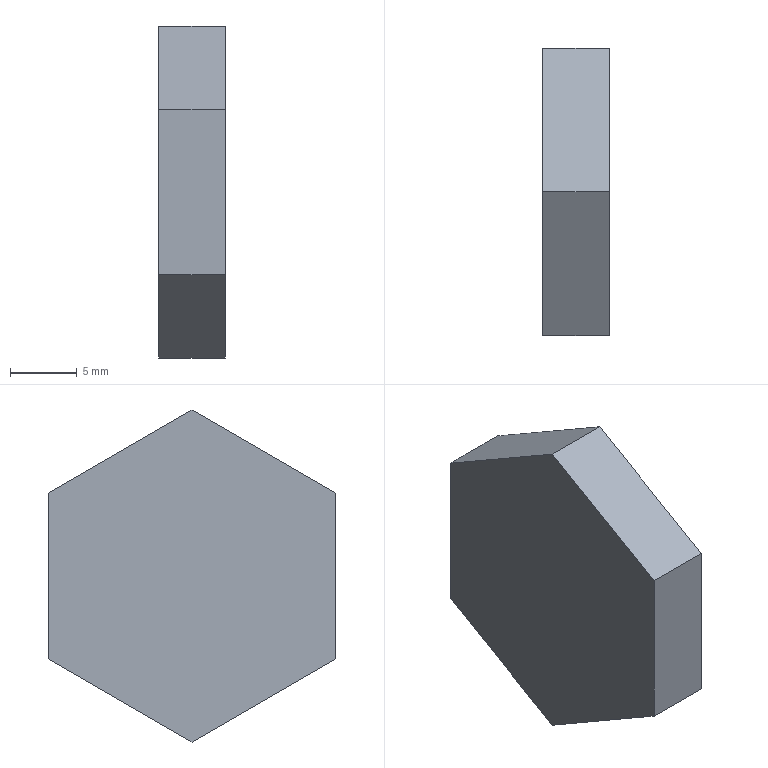Part | STEP file | 1 solid | 8 faces | box 5 x 21.5 x 24.826 mm | volume 2002 mm3 | plane 8
STEP:
#1=CARTESIAN_POINT('',(0.,0.,0.));
#2=DIRECTION('',(0.,0.,1.));
#3=DIRECTION('',(1.,0.,0.));
#4=AXIS2_PLACEMENT_3D('',#1,#2,#3);
#5=CARTESIAN_POINT('',(-24.,-10.75,6.207));
#6=VERTEX_POINT('',#5);
#7=CARTESIAN_POINT('',(-24.,-10.75,-6.207));
#8=VERTEX_POINT('',#7);
#9=CARTESIAN_POINT('',(-24.,-10.75,6.207));
#10=DIRECTION('',(0.,0.,-1.));
#11=VECTOR('',#10,1.);
#12=LINE('',#9,#11);
#13=CARTESIAN_POINT('',(-29.,-10.75,-3.464));
#14=DIRECTION('',(0.,1.,0.));
#15=DIRECTION('',(0.,0.,1.));
#16=AXIS2_PLACEMENT_3D('',#13,#14,#15);
#17=PLANE('',#16);
#18=CARTESIAN_POINT('',(9.671,5.));
#19=DIRECTION('',(-1.,0.));
#20=VECTOR('',#19,1.);
#21=LINE('',#18,#20);
#22=(GEOMETRIC_REPRESENTATION_CONTEXT(2)PARAMETRIC_REPRESENTATION_CONTEXT()REPRESENTATION_CONTEXT('',''));
#23=DEFINITIONAL_REPRESENTATION('',(#21),#22);
#24=PCURVE('',#17,#23);
#25=CARTESIAN_POINT('',(-24.,55.,0.));
#26=DIRECTION('',(-1.,0.,0.));
#27=DIRECTION('',(0.,0.,1.));
#28=AXIS2_PLACEMENT_3D('',#25,#26,#27);
#29=PLANE('',#28);
#30=CARTESIAN_POINT('',(6.207,-65.75));
#31=DIRECTION('',(-1.,0.));
#32=VECTOR('',#31,1.);
#33=LINE('',#30,#32);
#34=(GEOMETRIC_REPRESENTATION_CONTEXT(2)PARAMETRIC_REPRESENTATION_CONTEXT()REPRESENTATION_CONTEXT('',''));
#35=DEFINITIONAL_REPRESENTATION('',(#33),#34);
#36=PCURVE('',#29,#35);
#37=SURFACE_CURVE('',#12,(#24,#36),.PCURVE_S1.);
#38=EDGE_CURVE('',#6,#8,#37,.T.);
#39=ORIENTED_EDGE('',*,*,#38,.T.);
#40=CARTESIAN_POINT('',(-29.,-10.75,-6.207));
#41=VERTEX_POINT('',#40);
#42=CARTESIAN_POINT('',(-24.,-10.75,-6.207));
#43=DIRECTION('',(-1.,0.,0.));
#44=VECTOR('',#43,1.);
#45=LINE('',#42,#44);
#46=CARTESIAN_POINT('',(-2.742,5.));
#47=DIRECTION('',(0.,-1.));
#48=VECTOR('',#47,1.);
#49=LINE('',#46,#48);
#50=(GEOMETRIC_REPRESENTATION_CONTEXT(2)PARAMETRIC_REPRESENTATION_CONTEXT()REPRESENTATION_CONTEXT('',''));
#51=DEFINITIONAL_REPRESENTATION('',(#49),#50);
#52=PCURVE('',#17,#51);
#53=CARTESIAN_POINT('',(-29.,-2.375,-11.042));
#54=DIRECTION('',(0.,0.5,0.866));
#55=DIRECTION('',(0.,-0.866,0.5));
#56=AXIS2_PLACEMENT_3D('',#53,#54,#55);
#57=PLANE('',#56);
#58=CARTESIAN_POINT('',(9.671,5.));
#59=DIRECTION('',(0.,-1.));
#60=VECTOR('',#59,1.);
#61=LINE('',#58,#60);
#62=(GEOMETRIC_REPRESENTATION_CONTEXT(2)PARAMETRIC_REPRESENTATION_CONTEXT()REPRESENTATION_CONTEXT('',''));
#63=DEFINITIONAL_REPRESENTATION('',(#61),#62);
#64=PCURVE('',#57,#63);
#65=SURFACE_CURVE('',#45,(#52,#64),.PCURVE_S1.);
#66=EDGE_CURVE('',#8,#41,#65,.T.);
#67=ORIENTED_EDGE('',*,*,#66,.T.);
#68=CARTESIAN_POINT('',(-29.,-10.75,6.207));
#69=VERTEX_POINT('',#68);
#70=CARTESIAN_POINT('',(-29.,-10.75,6.207));
#71=DIRECTION('',(0.,0.,-1.));
#72=VECTOR('',#71,1.);
#73=LINE('',#70,#72);
#74=CARTESIAN_POINT('',(9.671,0.));
#75=DIRECTION('',(-1.,0.));
#76=VECTOR('',#75,1.);
#77=LINE('',#74,#76);
#78=(GEOMETRIC_REPRESENTATION_CONTEXT(2)PARAMETRIC_REPRESENTATION_CONTEXT()REPRESENTATION_CONTEXT('',''));
#79=DEFINITIONAL_REPRESENTATION('',(#77),#78);
#80=PCURVE('',#17,#79);
#81=CARTESIAN_POINT('',(-29.,55.,0.));
#82=DIRECTION('',(-1.,0.,0.));
#83=DIRECTION('',(0.,0.,1.));
#84=AXIS2_PLACEMENT_3D('',#81,#82,#83);
#85=PLANE('',#84);
#86=CARTESIAN_POINT('',(6.207,-65.75));
#87=DIRECTION('',(-1.,0.));
#88=VECTOR('',#87,1.);
#89=LINE('',#86,#88);
#90=(GEOMETRIC_REPRESENTATION_CONTEXT(2)PARAMETRIC_REPRESENTATION_CONTEXT()REPRESENTATION_CONTEXT('',''));
#91=DEFINITIONAL_REPRESENTATION('',(#89),#90);
#92=PCURVE('',#85,#91);
#93=SURFACE_CURVE('',#73,(#80,#92),.PCURVE_S1.);
#94=EDGE_CURVE('',#69,#41,#93,.T.);
#95=ORIENTED_EDGE('',*,*,#94,.F.);
#96=CARTESIAN_POINT('',(-24.,-10.75,6.207));
#97=DIRECTION('',(-1.,0.,0.));
#98=VECTOR('',#97,1.);
#99=LINE('',#96,#98);
#100=CARTESIAN_POINT('',(9.671,5.));
#101=DIRECTION('',(0.,-1.));
#102=VECTOR('',#101,1.);
#103=LINE('',#100,#102);
#104=(GEOMETRIC_REPRESENTATION_CONTEXT(2)PARAMETRIC_REPRESENTATION_CONTEXT()REPRESENTATION_CONTEXT('',''));
#105=DEFINITIONAL_REPRESENTATION('',(#103),#104);
#106=PCURVE('',#17,#105);
#107=CARTESIAN_POINT('',(-29.,-8.375,7.578));
#108=DIRECTION('',(0.,0.5,-0.866));
#109=DIRECTION('',(0.,0.866,0.5));
#110=AXIS2_PLACEMENT_3D('',#107,#108,#109);
#111=PLANE('',#110);
#112=CARTESIAN_POINT('',(-2.742,5.));
#113=DIRECTION('',(0.,-1.));
#114=VECTOR('',#113,1.);
#115=LINE('',#112,#114);
#116=(GEOMETRIC_REPRESENTATION_CONTEXT(2)PARAMETRIC_REPRESENTATION_CONTEXT()REPRESENTATION_CONTEXT('',''));
#117=DEFINITIONAL_REPRESENTATION('',(#115),#116);
#118=PCURVE('',#111,#117);
#119=SURFACE_CURVE('',#99,(#106,#118),.PCURVE_S1.);
#120=EDGE_CURVE('',#6,#69,#119,.T.);
#121=ORIENTED_EDGE('',*,*,#120,.F.);
#122=EDGE_LOOP('',(#39,#67,#95,#121));
#123=FACE_BOUND('',#122,.F.);
#124=ADVANCED_FACE('',(#123),#17,.F.);
#125=ORIENTED_EDGE('',*,*,#38,.F.);
#126=CARTESIAN_POINT('',(-24.,0.,12.413));
#127=VERTEX_POINT('',#126);
#128=CARTESIAN_POINT('',(-24.,0.,12.413));
#129=DIRECTION('',(0.,-0.866,-0.5));
#130=VECTOR('',#129,1.);
#131=LINE('',#128,#130);
#132=CARTESIAN_POINT('',(12.413,-55.));
#133=DIRECTION('',(-0.5,-0.866));
#134=VECTOR('',#133,1.);
#135=LINE('',#132,#134);
#136=(GEOMETRIC_REPRESENTATION_CONTEXT(2)PARAMETRIC_REPRESENTATION_CONTEXT()REPRESENTATION_CONTEXT('',''));
#137=DEFINITIONAL_REPRESENTATION('',(#135),#136);
#138=PCURVE('',#29,#137);
#139=CARTESIAN_POINT('',(9.671,5.));
#140=DIRECTION('',(-1.,0.));
#141=VECTOR('',#140,1.);
#142=LINE('',#139,#141);
#143=(GEOMETRIC_REPRESENTATION_CONTEXT(2)PARAMETRIC_REPRESENTATION_CONTEXT()REPRESENTATION_CONTEXT('',''));
#144=DEFINITIONAL_REPRESENTATION('',(#142),#143);
#145=PCURVE('',#111,#144);
#146=SURFACE_CURVE('',#131,(#138,#145),.PCURVE_S1.);
#147=EDGE_CURVE('',#127,#6,#146,.T.);
#148=ORIENTED_EDGE('',*,*,#147,.F.);
#149=CARTESIAN_POINT('',(-24.,10.75,6.207));
#150=VERTEX_POINT('',#149);
#151=CARTESIAN_POINT('',(-24.,10.75,6.207));
#152=DIRECTION('',(0.,-0.866,0.5));
#153=VECTOR('',#152,1.);
#154=LINE('',#151,#153);
#155=CARTESIAN_POINT('',(6.207,-44.25));
#156=DIRECTION('',(0.5,-0.866));
#157=VECTOR('',#156,1.);
#158=LINE('',#155,#157);
#159=(GEOMETRIC_REPRESENTATION_CONTEXT(2)PARAMETRIC_REPRESENTATION_CONTEXT()REPRESENTATION_CONTEXT('',''));
#160=DEFINITIONAL_REPRESENTATION('',(#158),#159);
#161=PCURVE('',#29,#160);
#162=CARTESIAN_POINT('',(-29.,2.375,11.042));
#163=DIRECTION('',(0.,-0.5,-0.866));
#164=DIRECTION('',(0.,0.866,-0.5));
#165=AXIS2_PLACEMENT_3D('',#162,#163,#164);
#166=PLANE('',#165);
#167=CARTESIAN_POINT('',(9.671,5.));
#168=DIRECTION('',(-1.,0.));
#169=VECTOR('',#168,1.);
#170=LINE('',#167,#169);
#171=(GEOMETRIC_REPRESENTATION_CONTEXT(2)PARAMETRIC_REPRESENTATION_CONTEXT()REPRESENTATION_CONTEXT('',''));
#172=DEFINITIONAL_REPRESENTATION('',(#170),#171);
#173=PCURVE('',#166,#172);
#174=SURFACE_CURVE('',#154,(#161,#173),.PCURVE_S1.);
#175=EDGE_CURVE('',#150,#127,#174,.T.);
#176=ORIENTED_EDGE('',*,*,#175,.F.);
#177=CARTESIAN_POINT('',(-24.,10.75,-6.207));
#178=VERTEX_POINT('',#177);
#179=CARTESIAN_POINT('',(-24.,10.75,-6.207));
#180=DIRECTION('',(0.,0.,1.));
#181=VECTOR('',#180,1.);
#182=LINE('',#179,#181);
#183=CARTESIAN_POINT('',(-6.207,-44.25));
#184=DIRECTION('',(1.,0.));
#185=VECTOR('',#184,1.);
#186=LINE('',#183,#185);
#187=(GEOMETRIC_REPRESENTATION_CONTEXT(2)PARAMETRIC_REPRESENTATION_CONTEXT()REPRESENTATION_CONTEXT('',''));
#188=DEFINITIONAL_REPRESENTATION('',(#186),#187);
#189=PCURVE('',#29,#188);
#190=CARTESIAN_POINT('',(-29.,10.75,3.464));
#191=DIRECTION('',(0.,-1.,0.));
#192=DIRECTION('',(0.,0.,-1.));
#193=AXIS2_PLACEMENT_3D('',#190,#191,#192);
#194=PLANE('',#193);
#195=CARTESIAN_POINT('',(9.671,5.));
#196=DIRECTION('',(-1.,0.));
#197=VECTOR('',#196,1.);
#198=LINE('',#195,#197);
#199=(GEOMETRIC_REPRESENTATION_CONTEXT(2)PARAMETRIC_REPRESENTATION_CONTEXT()REPRESENTATION_CONTEXT('',''));
#200=DEFINITIONAL_REPRESENTATION('',(#198),#199);
#201=PCURVE('',#194,#200);
#202=SURFACE_CURVE('',#182,(#189,#201),.PCURVE_S1.);
#203=EDGE_CURVE('',#178,#150,#202,.T.);
#204=ORIENTED_EDGE('',*,*,#203,.F.);
#205=CARTESIAN_POINT('',(-24.,0.,-12.413));
#206=VERTEX_POINT('',#205);
#207=CARTESIAN_POINT('',(-24.,0.,-12.413));
#208=DIRECTION('',(0.,0.866,0.5));
#209=VECTOR('',#208,1.);
#210=LINE('',#207,#209);
#211=CARTESIAN_POINT('',(-12.413,-55.));
#212=DIRECTION('',(0.5,0.866));
#213=VECTOR('',#212,1.);
#214=LINE('',#211,#213);
#215=(GEOMETRIC_REPRESENTATION_CONTEXT(2)PARAMETRIC_REPRESENTATION_CONTEXT()REPRESENTATION_CONTEXT('',''));
#216=DEFINITIONAL_REPRESENTATION('',(#214),#215);
#217=PCURVE('',#29,#216);
#218=CARTESIAN_POINT('',(-29.,8.375,-7.578));
#219=DIRECTION('',(0.,-0.5,0.866));
#220=DIRECTION('',(0.,-0.866,-0.5));
#221=AXIS2_PLACEMENT_3D('',#218,#219,#220);
#222=PLANE('',#221);
#223=CARTESIAN_POINT('',(9.671,5.));
#224=DIRECTION('',(-1.,0.));
#225=VECTOR('',#224,1.);
#226=LINE('',#223,#225);
#227=(GEOMETRIC_REPRESENTATION_CONTEXT(2)PARAMETRIC_REPRESENTATION_CONTEXT()REPRESENTATION_CONTEXT('',''));
#228=DEFINITIONAL_REPRESENTATION('',(#226),#227);
#229=PCURVE('',#222,#228);
#230=SURFACE_CURVE('',#210,(#217,#229),.PCURVE_S1.);
#231=EDGE_CURVE('',#206,#178,#230,.T.);
#232=ORIENTED_EDGE('',*,*,#231,.F.);
#233=CARTESIAN_POINT('',(-24.,-10.75,-6.207));
#234=DIRECTION('',(0.,0.866,-0.5));
#235=VECTOR('',#234,1.);
#236=LINE('',#233,#235);
#237=CARTESIAN_POINT('',(-6.207,-65.75));
#238=DIRECTION('',(-0.5,0.866));
#239=VECTOR('',#238,1.);
#240=LINE('',#237,#239);
#241=(GEOMETRIC_REPRESENTATION_CONTEXT(2)PARAMETRIC_REPRESENTATION_CONTEXT()REPRESENTATION_CONTEXT('',''));
#242=DEFINITIONAL_REPRESENTATION('',(#240),#241);
#243=PCURVE('',#29,#242);
#244=CARTESIAN_POINT('',(9.671,5.));
#245=DIRECTION('',(-1.,0.));
#246=VECTOR('',#245,1.);
#247=LINE('',#244,#246);
#248=(GEOMETRIC_REPRESENTATION_CONTEXT(2)PARAMETRIC_REPRESENTATION_CONTEXT()REPRESENTATION_CONTEXT('',''));
#249=DEFINITIONAL_REPRESENTATION('',(#247),#248);
#250=PCURVE('',#57,#249);
#251=SURFACE_CURVE('',#236,(#243,#250),.PCURVE_S1.);
#252=EDGE_CURVE('',#8,#206,#251,.T.);
#253=ORIENTED_EDGE('',*,*,#252,.F.);
#254=EDGE_LOOP('',(#125,#148,#176,#204,#232,#253));
#255=FACE_BOUND('',#254,.F.);
#256=ADVANCED_FACE('',(#255),#29,.F.);
#257=ORIENTED_EDGE('',*,*,#147,.T.);
#258=ORIENTED_EDGE('',*,*,#120,.T.);
#259=CARTESIAN_POINT('',(-29.,0.,12.413));
#260=VERTEX_POINT('',#259);
#261=CARTESIAN_POINT('',(-29.,-10.75,6.207));
#262=DIRECTION('',(0.,0.866,0.5));
#263=VECTOR('',#262,1.);
#264=LINE('',#261,#263);
#265=CARTESIAN_POINT('',(-2.742,0.));
#266=DIRECTION('',(1.,0.));
#267=VECTOR('',#266,1.);
#268=LINE('',#265,#267);
#269=(GEOMETRIC_REPRESENTATION_CONTEXT(2)PARAMETRIC_REPRESENTATION_CONTEXT()REPRESENTATION_CONTEXT('',''));
#270=DEFINITIONAL_REPRESENTATION('',(#268),#269);
#271=PCURVE('',#111,#270);
#272=CARTESIAN_POINT('',(6.207,-65.75));
#273=DIRECTION('',(0.5,0.866));
#274=VECTOR('',#273,1.);
#275=LINE('',#272,#274);
#276=(GEOMETRIC_REPRESENTATION_CONTEXT(2)PARAMETRIC_REPRESENTATION_CONTEXT()REPRESENTATION_CONTEXT('',''));
#277=DEFINITIONAL_REPRESENTATION('',(#275),#276);
#278=PCURVE('',#85,#277);
#279=SURFACE_CURVE('',#264,(#271,#278),.PCURVE_S1.);
#280=EDGE_CURVE('',#69,#260,#279,.T.);
#281=ORIENTED_EDGE('',*,*,#280,.T.);
#282=CARTESIAN_POINT('',(-24.,0.,12.413));
#283=DIRECTION('',(-1.,0.,0.));
#284=VECTOR('',#283,1.);
#285=LINE('',#282,#284);
#286=CARTESIAN_POINT('',(9.671,5.));
#287=DIRECTION('',(0.,-1.));
#288=VECTOR('',#287,1.);
#289=LINE('',#286,#288);
#290=(GEOMETRIC_REPRESENTATION_CONTEXT(2)PARAMETRIC_REPRESENTATION_CONTEXT()REPRESENTATION_CONTEXT('',''));
#291=DEFINITIONAL_REPRESENTATION('',(#289),#290);
#292=PCURVE('',#111,#291);
#293=CARTESIAN_POINT('',(-2.742,5.));
#294=DIRECTION('',(0.,-1.));
#295=VECTOR('',#294,1.);
#296=LINE('',#293,#295);
#297=(GEOMETRIC_REPRESENTATION_CONTEXT(2)PARAMETRIC_REPRESENTATION_CONTEXT()REPRESENTATION_CONTEXT('',''));
#298=DEFINITIONAL_REPRESENTATION('',(#296),#297);
#299=PCURVE('',#166,#298);
#300=SURFACE_CURVE('',#285,(#292,#299),.PCURVE_S1.);
#301=EDGE_CURVE('',#127,#260,#300,.T.);
#302=ORIENTED_EDGE('',*,*,#301,.F.);
#303=EDGE_LOOP('',(#257,#258,#281,#302));
#304=FACE_BOUND('',#303,.F.);
#305=ADVANCED_FACE('',(#304),#111,.F.);
#306=ORIENTED_EDGE('',*,*,#94,.T.);
#307=CARTESIAN_POINT('',(-29.,0.,-12.413));
#308=VERTEX_POINT('',#307);
#309=CARTESIAN_POINT('',(-29.,0.,-12.413));
#310=DIRECTION('',(0.,-0.866,0.5));
#311=VECTOR('',#310,1.);
#312=LINE('',#309,#311);
#313=CARTESIAN_POINT('',(-12.413,-55.));
#314=DIRECTION('',(0.5,-0.866));
#315=VECTOR('',#314,1.);
#316=LINE('',#313,#315);
#317=(GEOMETRIC_REPRESENTATION_CONTEXT(2)PARAMETRIC_REPRESENTATION_CONTEXT()REPRESENTATION_CONTEXT('',''));
#318=DEFINITIONAL_REPRESENTATION('',(#316),#317);
#319=PCURVE('',#85,#318);
#320=CARTESIAN_POINT('',(-2.742,0.));
#321=DIRECTION('',(1.,0.));
#322=VECTOR('',#321,1.);
#323=LINE('',#320,#322);
#324=(GEOMETRIC_REPRESENTATION_CONTEXT(2)PARAMETRIC_REPRESENTATION_CONTEXT()REPRESENTATION_CONTEXT('',''));
#325=DEFINITIONAL_REPRESENTATION('',(#323),#324);
#326=PCURVE('',#57,#325);
#327=SURFACE_CURVE('',#312,(#319,#326),.PCURVE_S1.);
#328=EDGE_CURVE('',#308,#41,#327,.T.);
#329=ORIENTED_EDGE('',*,*,#328,.F.);
#330=CARTESIAN_POINT('',(-29.,10.75,-6.207));
#331=VERTEX_POINT('',#330);
#332=CARTESIAN_POINT('',(-29.,10.75,-6.207));
#333=DIRECTION('',(0.,-0.866,-0.5));
#334=VECTOR('',#333,1.);
#335=LINE('',#332,#334);
#336=CARTESIAN_POINT('',(-6.207,-44.25));
#337=DIRECTION('',(-0.5,-0.866));
#338=VECTOR('',#337,1.);
#339=LINE('',#336,#338);
#340=(GEOMETRIC_REPRESENTATION_CONTEXT(2)PARAMETRIC_REPRESENTATION_CONTEXT()REPRESENTATION_CONTEXT('',''));
#341=DEFINITIONAL_REPRESENTATION('',(#339),#340);
#342=PCURVE('',#85,#341);
#343=CARTESIAN_POINT('',(-2.742,0.));
#344=DIRECTION('',(1.,0.));
#345=VECTOR('',#344,1.);
#346=LINE('',#343,#345);
#347=(GEOMETRIC_REPRESENTATION_CONTEXT(2)PARAMETRIC_REPRESENTATION_CONTEXT()REPRESENTATION_CONTEXT('',''));
#348=DEFINITIONAL_REPRESENTATION('',(#346),#347);
#349=PCURVE('',#222,#348);
#350=SURFACE_CURVE('',#335,(#342,#349),.PCURVE_S1.);
#351=EDGE_CURVE('',#331,#308,#350,.T.);
#352=ORIENTED_EDGE('',*,*,#351,.F.);
#353=CARTESIAN_POINT('',(-29.,10.75,6.207));
#354=VERTEX_POINT('',#353);
#355=CARTESIAN_POINT('',(-29.,10.75,-6.207));
#356=DIRECTION('',(0.,0.,1.));
#357=VECTOR('',#356,1.);
#358=LINE('',#355,#357);
#359=CARTESIAN_POINT('',(-6.207,-44.25));
#360=DIRECTION('',(1.,0.));
#361=VECTOR('',#360,1.);
#362=LINE('',#359,#361);
#363=(GEOMETRIC_REPRESENTATION_CONTEXT(2)PARAMETRIC_REPRESENTATION_CONTEXT()REPRESENTATION_CONTEXT('',''));
#364=DEFINITIONAL_REPRESENTATION('',(#362),#363);
#365=PCURVE('',#85,#364);
#366=CARTESIAN_POINT('',(9.671,0.));
#367=DIRECTION('',(-1.,0.));
#368=VECTOR('',#367,1.);
#369=LINE('',#366,#368);
#370=(GEOMETRIC_REPRESENTATION_CONTEXT(2)PARAMETRIC_REPRESENTATION_CONTEXT()REPRESENTATION_CONTEXT('',''));
#371=DEFINITIONAL_REPRESENTATION('',(#369),#370);
#372=PCURVE('',#194,#371);
#373=SURFACE_CURVE('',#358,(#365,#372),.PCURVE_S1.);
#374=EDGE_CURVE('',#331,#354,#373,.T.);
#375=ORIENTED_EDGE('',*,*,#374,.T.);
#376=CARTESIAN_POINT('',(-29.,0.,12.413));
#377=DIRECTION('',(0.,0.866,-0.5));
#378=VECTOR('',#377,1.);
#379=LINE('',#376,#378);
#380=CARTESIAN_POINT('',(12.413,-55.));
#381=DIRECTION('',(-0.5,0.866));
#382=VECTOR('',#381,1.);
#383=LINE('',#380,#382);
#384=(GEOMETRIC_REPRESENTATION_CONTEXT(2)PARAMETRIC_REPRESENTATION_CONTEXT()REPRESENTATION_CONTEXT('',''));
#385=DEFINITIONAL_REPRESENTATION('',(#383),#384);
#386=PCURVE('',#85,#385);
#387=CARTESIAN_POINT('',(-2.742,0.));
#388=DIRECTION('',(1.,0.));
#389=VECTOR('',#388,1.);
#390=LINE('',#387,#389);
#391=(GEOMETRIC_REPRESENTATION_CONTEXT(2)PARAMETRIC_REPRESENTATION_CONTEXT()REPRESENTATION_CONTEXT('',''));
#392=DEFINITIONAL_REPRESENTATION('',(#390),#391);
#393=PCURVE('',#166,#392);
#394=SURFACE_CURVE('',#379,(#386,#393),.PCURVE_S1.);
#395=EDGE_CURVE('',#260,#354,#394,.T.);
#396=ORIENTED_EDGE('',*,*,#395,.F.);
#397=ORIENTED_EDGE('',*,*,#280,.F.);
#398=EDGE_LOOP('',(#306,#329,#352,#375,#396,#397));
#399=FACE_BOUND('',#398,.F.);
#400=ADVANCED_FACE('',(#399),#85,.T.);
#401=ORIENTED_EDGE('',*,*,#252,.T.);
#402=CARTESIAN_POINT('',(-24.,0.,-12.413));
#403=DIRECTION('',(-1.,0.,0.));
#404=VECTOR('',#403,1.);
#405=LINE('',#402,#404);
#406=CARTESIAN_POINT('',(-2.742,5.));
#407=DIRECTION('',(0.,-1.));
#408=VECTOR('',#407,1.);
#409=LINE('',#406,#408);
#410=(GEOMETRIC_REPRESENTATION_CONTEXT(2)PARAMETRIC_REPRESENTATION_CONTEXT()REPRESENTATION_CONTEXT('',''));
#411=DEFINITIONAL_REPRESENTATION('',(#409),#410);
#412=PCURVE('',#57,#411);
#413=CARTESIAN_POINT('',(9.671,5.));
#414=DIRECTION('',(0.,-1.));
#415=VECTOR('',#414,1.);
#416=LINE('',#413,#415);
#417=(GEOMETRIC_REPRESENTATION_CONTEXT(2)PARAMETRIC_REPRESENTATION_CONTEXT()REPRESENTATION_CONTEXT('',''));
#418=DEFINITIONAL_REPRESENTATION('',(#416),#417);
#419=PCURVE('',#222,#418);
#420=SURFACE_CURVE('',#405,(#412,#419),.PCURVE_S1.);
#421=EDGE_CURVE('',#206,#308,#420,.T.);
#422=ORIENTED_EDGE('',*,*,#421,.T.);
#423=ORIENTED_EDGE('',*,*,#328,.T.);
#424=ORIENTED_EDGE('',*,*,#66,.F.);
#425=EDGE_LOOP('',(#401,#422,#423,#424));
#426=FACE_BOUND('',#425,.F.);
#427=ADVANCED_FACE('',(#426),#57,.F.);
#428=ORIENTED_EDGE('',*,*,#231,.T.);
#429=CARTESIAN_POINT('',(-24.,10.75,-6.207));
#430=DIRECTION('',(-1.,0.,0.));
#431=VECTOR('',#430,1.);
#432=LINE('',#429,#431);
#433=CARTESIAN_POINT('',(-2.742,5.));
#434=DIRECTION('',(0.,-1.));
#435=VECTOR('',#434,1.);
#436=LINE('',#433,#435);
#437=(GEOMETRIC_REPRESENTATION_CONTEXT(2)PARAMETRIC_REPRESENTATION_CONTEXT()REPRESENTATION_CONTEXT('',''));
#438=DEFINITIONAL_REPRESENTATION('',(#436),#437);
#439=PCURVE('',#222,#438);
#440=CARTESIAN_POINT('',(9.671,5.));
#441=DIRECTION('',(0.,-1.));
#442=VECTOR('',#441,1.);
#443=LINE('',#440,#442);
#444=(GEOMETRIC_REPRESENTATION_CONTEXT(2)PARAMETRIC_REPRESENTATION_CONTEXT()REPRESENTATION_CONTEXT('',''));
#445=DEFINITIONAL_REPRESENTATION('',(#443),#444);
#446=PCURVE('',#194,#445);
#447=SURFACE_CURVE('',#432,(#439,#446),.PCURVE_S1.);
#448=EDGE_CURVE('',#178,#331,#447,.T.);
#449=ORIENTED_EDGE('',*,*,#448,.T.);
#450=ORIENTED_EDGE('',*,*,#351,.T.);
#451=ORIENTED_EDGE('',*,*,#421,.F.);
#452=EDGE_LOOP('',(#428,#449,#450,#451));
#453=FACE_BOUND('',#452,.F.);
#454=ADVANCED_FACE('',(#453),#222,.F.);
#455=ORIENTED_EDGE('',*,*,#203,.T.);
#456=CARTESIAN_POINT('',(-24.,10.75,6.207));
#457=DIRECTION('',(-1.,0.,0.));
#458=VECTOR('',#457,1.);
#459=LINE('',#456,#458);
#460=CARTESIAN_POINT('',(-2.742,5.));
#461=DIRECTION('',(0.,-1.));
#462=VECTOR('',#461,1.);
#463=LINE('',#460,#462);
#464=(GEOMETRIC_REPRESENTATION_CONTEXT(2)PARAMETRIC_REPRESENTATION_CONTEXT()REPRESENTATION_CONTEXT('',''));
#465=DEFINITIONAL_REPRESENTATION('',(#463),#464);
#466=PCURVE('',#194,#465);
#467=CARTESIAN_POINT('',(9.671,5.));
#468=DIRECTION('',(0.,-1.));
#469=VECTOR('',#468,1.);
#470=LINE('',#467,#469);
#471=(GEOMETRIC_REPRESENTATION_CONTEXT(2)PARAMETRIC_REPRESENTATION_CONTEXT()REPRESENTATION_CONTEXT('',''));
#472=DEFINITIONAL_REPRESENTATION('',(#470),#471);
#473=PCURVE('',#166,#472);
#474=SURFACE_CURVE('',#459,(#466,#473),.PCURVE_S1.);
#475=EDGE_CURVE('',#150,#354,#474,.T.);
#476=ORIENTED_EDGE('',*,*,#475,.T.);
#477=ORIENTED_EDGE('',*,*,#374,.F.);
#478=ORIENTED_EDGE('',*,*,#448,.F.);
#479=EDGE_LOOP('',(#455,#476,#477,#478));
#480=FACE_BOUND('',#479,.F.);
#481=ADVANCED_FACE('',(#480),#194,.F.);
#482=ORIENTED_EDGE('',*,*,#175,.T.);
#483=ORIENTED_EDGE('',*,*,#301,.T.);
#484=ORIENTED_EDGE('',*,*,#395,.T.);
#485=ORIENTED_EDGE('',*,*,#475,.F.);
#486=EDGE_LOOP('',(#482,#483,#484,#485));
#487=FACE_BOUND('',#486,.F.);
#488=ADVANCED_FACE('',(#487),#166,.F.);
#489=CLOSED_SHELL('',(#124,#256,#305,#400,#427,#454,#481,#488));
#490=MANIFOLD_SOLID_BREP('',#489);
#491=(LENGTH_UNIT()NAMED_UNIT(*)SI_UNIT(.MILLI.,.METRE.));
#492=UNCERTAINTY_MEASURE_WITH_UNIT(LENGTH_MEASURE(0.0000001),#491,'','');
#493=(NAMED_UNIT(*)PLANE_ANGLE_UNIT()SI_UNIT($,.RADIAN.));
#494=(NAMED_UNIT(*)SI_UNIT($,.STERADIAN.)SOLID_ANGLE_UNIT());
#495=(GEOMETRIC_REPRESENTATION_CONTEXT(3)GLOBAL_UNCERTAINTY_ASSIGNED_CONTEXT((#492))GLOBAL_UNIT_ASSIGNED_CONTEXT((#491,#493,#494))REPRESENTATION_CONTEXT('',''));
#496=ADVANCED_BREP_SHAPE_REPRESENTATION('',(#4,#490),#495);